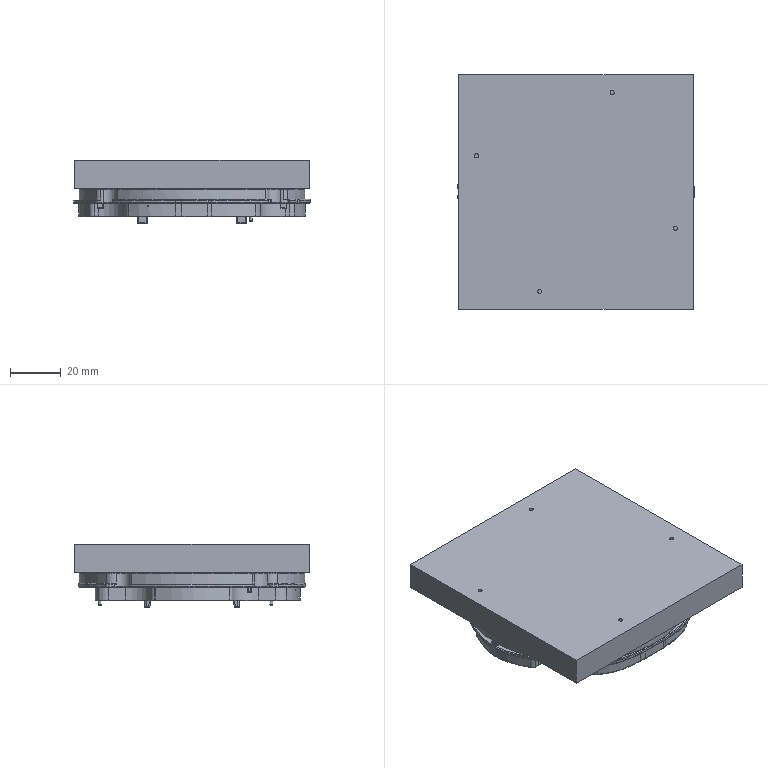NC program | NX | posted with a generic post | part box 92.935 x 92.1 x 24.829 mm
Lines 11819 to 12564 of 39008:
(ADAPTIVE_MILLING_COPY , TOOL : D3-9-D4-50-3T-ROUGH)
N23624 T15 M6
N23626 G54
N23628 G17 G0 G90 X32.559 Y-28.253 S5500 M3
N23630 G43 Z20. H15
N23632 Z-4.875
N23634 G94 G1 X32.611 Y-28.113 Z-5.812 F3000.
N23636 X32.662 Y-27.972 Z-6.183
N23638 X32.714 Y-27.831 Z-6.456
N23640 X32.765 Y-27.69 Z-6.675
N23642 X32.817 Y-27.549 Z-6.86
N23644 X32.868 Y-27.408 Z-7.018
N23646 X32.92 Y-27.267 Z-7.155
N23648 X32.971 Y-27.126 Z-7.275
N23650 X33.023 Y-26.986 Z-7.381
N23652 X33.074 Y-26.845 Z-7.474
N23654 X33.126 Y-26.704 Z-7.555
N23656 X33.177 Y-26.563 Z-7.625
N23658 X33.229 Y-26.422 Z-7.686
N23660 X33.28 Y-26.281 Z-7.737
N23662 X33.332 Y-26.14 Z-7.78
N23664 X33.383 Y-25.999 Z-7.815
N23666 X33.435 Y-25.858 Z-7.842
N23668 X33.486 Y-25.718 Z-7.86
N23670 X33.538 Y-25.577 Z-7.872
N23672 X33.589 Y-25.436 Z-7.875
N23674 X33.692 Y-25.162
N23676 X33.783 Y-24.884
N23678 G3 X33.696 Y-24.632 R0.309
N23680 X31.619 Y-23.863 R2.562
N23682 X28.424 Y-26.256 R3.555
N23684 G1 Y-26.893
N23686 G3 X28.606 Y-27.188 R0.332
N23688 X28.976 Y-27.152 Z-7.809 R0.385
N23690 G1 X29.156 Y-27.065 Z-7.775
N23692 X33.131 Y-25.119 F15000.
N23694 X33.313 Y-25.032 Z-7.81 F3000.
N23696 X33.488 Y-24.932 Z-7.844
N23698 X33.55 Y-24.863 Z-7.86
N23700 X33.591 Y-24.781 Z-7.875
N23702 G3 X33.511 Y-24.446 R0.332
N23704 X31.622 Y-23.664 R2.242
N23706 X28.444 Y-25.702 R3.596
N23708 G1 X28.424 Y-26.264
N23710 G3 X28.601 Y-26.556 R0.332
N23712 X28.967 Y-26.532 Z-7.811 R0.391
N23714 G1 X29.156 Y-26.449 Z-7.775
N23716 X32.857 Y-24.844 F15000.
N23718 X33.045 Y-24.764 Z-7.81 F3000.
N23720 X33.227 Y-24.672 Z-7.845
N23722 X33.29 Y-24.608 Z-7.86
N23724 X33.336 Y-24.531 Z-7.875
N23726 G3 X33.323 Y-24.259 R0.337
N23728 X32.298 Y-23.553 R1.442
N23730 X28.496 Y-25.188 R3.657
N23732 G1 X28.442 Y-25.733
N23734 G3 X28.594 Y-26.038 R0.332
N23736 X28.961 Y-26.042 Z-7.81 R0.39
N23738 G1 X29.156 Y-25.975 Z-7.775
N23740 X32.755 Y-24.735 F15000.
N23742 X32.955 Y-24.668 Z-7.811 F3000.
N23744 X33.15 Y-24.589 Z-7.847
N23746 X33.215 Y-24.536 Z-7.861
N23748 X33.266 Y-24.47 Z-7.875
N23750 G3 X33.272 Y-24.159 R0.334
N23752 X32.215 Y-23.363 R1.429
N23754 X28.532 Y-24.788 R3.673
N23756 G1 X28.478 Y-25.273
N23758 G3 X28.627 Y-25.575 R0.333
N23760 X28.979 Y-25.592 Z-7.813 R0.387
N23762 G1 X29.192 Y-25.53 Z-7.775
N23764 X32.625 Y-24.526 F15000.
N23766 X32.831 Y-24.467 Z-7.812 F3000.
N23768 X33.033 Y-24.398 Z-7.848
N23770 X33.097 Y-24.35 Z-7.862
N23772 X33.151 Y-24.29 Z-7.875
N23774 G3 X33.17 Y-23.959 R0.333
N23776 X32.084 Y-23.163 R1.454
N23778 X28.602 Y-24.38 R3.693
N23780 X28.51 Y-24.866 R2.637
N23782 X28.656 Y-25.166 R0.333
N23784 X29. Y-25.192 Z-7.815 R0.396
N23786 G1 X29.224 Y-25.138 Z-7.775
N23788 X32.533 Y-24.343 F15000.
N23790 X32.736 Y-24.296 Z-7.811 F3000.
N23792 X32.937 Y-24.236 Z-7.847
N23794 X33.007 Y-24.188 Z-7.861
N23796 X33.065 Y-24.126 Z-7.875
N23798 G3 X33.085 Y-23.791 R0.333
N23800 X32.027 Y-22.98 R1.401
N23802 X28.709 Y-23.971 R3.668
N23804 G1 X28.576 Y-24.446
N23806 G3 X28.686 Y-24.777 R0.332
N23808 X29.041 Y-24.831 Z-7.812 R0.382
N23810 G1 X29.252 Y-24.788 Z-7.775
N23812 X32.435 Y-24.153 F15000.
N23814 X32.643 Y-24.113 Z-7.811 F3000.
N23816 X32.849 Y-24.062 Z-7.848
N23818 X32.919 Y-24.019 Z-7.861
N23820 X32.978 Y-23.962 Z-7.875
N23822 G3 X33.043 Y-23.709 R0.339
N23824 X32.37 Y-22.942 R1.058
N23826 X29.652 Y-23.059 R3.291
N23828 X28.772 Y-23.665 R2.172
N23830 G1 X28.666 Y-24.071
N23832 G3 X28.766 Y-24.394 R0.333
N23834 X29.113 Y-24.464 Z-7.813 R0.386
N23836 G1 X29.332 Y-24.435 Z-7.775
N23838 X32.373 Y-24.026 F15000.
N23840 X32.598 Y-23.999 Z-7.814 F3000.
N23842 X32.821 Y-23.955 Z-7.853
N23844 X32.933 Y-23.882 Z-7.875
N23846 G3 X33.025 Y-23.598 R0.334
N23848 X32.262 Y-22.73 R1.156
N23850 X28.885 Y-23.292 R3.407
N23852 X28.746 Y-23.74 R1.548
N23854 X28.842 Y-24.059 R0.333
N23856 X29.178 Y-24.139 Z-7.815 R0.396
N23858 G1 X29.408 Y-24.121 Z-7.775
N23860 X32.327 Y-23.896 F15000.
N23862 X32.556 Y-23.882 Z-7.814 F3000.
N23864 X32.783 Y-23.851 Z-7.854
N23866 X32.896 Y-23.789 Z-7.875
N23868 G3 X33.008 Y-23.486 R0.333
N23870 X32.259 Y-22.565 R1.163
N23872 X29.043 Y-22.925 R3.351
N23874 X28.828 Y-23.4 R4.539
N23876 X28.918 Y-23.733 R0.319
N23878 X29.229 Y-23.811 Z-7.819 R0.389
N23880 G1 X29.486 Y-23.8 Z-7.775
N23882 X32.287 Y-23.684 F15000.
N23884 X32.52 Y-23.677 Z-7.815 F3000.
N23886 X32.751 Y-23.655 Z-7.855
N23888 X32.861 Y-23.6 Z-7.875
N23890 G3 X32.978 Y-23.301 R0.32
N23892 X32.217 Y-22.377 R1.206
N23894 X29.175 Y-22.613 R3.245
N23896 X28.99 Y-23.002 R3.691
N23898 X29.038 Y-23.336 R0.333
N23900 X29.37 Y-23.46 Z-7.813 R0.386
N23902 G1 X29.59 Y-23.465 Z-7.775
N23904 X32.262 Y-23.526 F15000.
N23906 X32.476 Y-23.533 Z-7.812 F3000.
N23908 X32.69 Y-23.528 Z-7.848
N23910 X32.766 Y-23.503 Z-7.862
N23912 X32.835 Y-23.463 Z-7.875
N23914 G3 X32.955 Y-23.153 R0.333
N23916 X32.258 Y-22.229 R1.165
N23918 X29.304 Y-22.319 R3.114
N23920 X29.106 Y-22.721 R1.623
N23922 X29.152 Y-23.052 R0.333
N23924 X29.474 Y-23.182 Z-7.814 R0.393
N23926 G1 X29.702 Y-23.197 Z-7.775
N23928 X32.237 Y-23.366 F15000.
N23930 X32.45 Y-23.382 Z-7.812 F3000.
N23932 X32.663 Y-23.387 Z-7.848
N23934 X32.741 Y-23.364 Z-7.862
N23936 X32.812 Y-23.327 Z-7.875
N23938 G3 X32.946 Y-23.061 R0.335
N23940 X32.403 Y-22.149 R1.061
N23942 X29.455 Y-22.026 R3.026
N23944 X29.233 Y-22.415 R0.964
N23946 X29.276 Y-22.743 R0.333
N23948 X29.58 Y-22.879 Z-7.817 R0.393
N23950 G1 X29.823 Y-22.908 Z-7.775
N23952 X32.212 Y-23.195 F15000.
N23954 X32.438 Y-23.225 Z-7.814 F3000.
N23956 X32.665 Y-23.237 Z-7.853
N23958 X32.789 Y-23.192 Z-7.875
N23960 G3 X32.946 Y-22.911 R0.333
N23962 X32.373 Y-21.954 R1.113
N23964 X29.613 Y-21.755 R2.886
N23966 G1 X29.378 Y-22.103
N23968 G3 X29.389 Y-22.465 R0.332
N23970 X29.687 Y-22.614 Z-7.817 R0.392
N23972 G1 X29.928 Y-22.654 Z-7.775
N23974 X32.203 Y-23.027 F15000.
N23976 X32.416 Y-23.064 Z-7.812 F3000.
N23978 X32.63 Y-23.09 Z-7.849
N23980 X32.707 Y-23.076 Z-7.862
N23982 X32.78 Y-23.047 Z-7.875
N23984 G3 X32.946 Y-22.761 R0.333
N23986 X32.363 Y-21.77 R1.152
N23988 X29.804 Y-21.477 R2.856
N23990 X29.551 Y-21.821 R1.132
N23992 X29.544 Y-22.154 R0.333
N23994 X29.844 Y-22.334 Z-7.814 R0.391
N23996 G1 X30.065 Y-22.383 Z-7.775
N23998 X32.204 Y-22.857 F15000.
N24000 X32.409 Y-22.905 Z-7.811 F3000.
N24002 X32.616 Y-22.94 Z-7.847
N24004 X32.699 Y-22.928 Z-7.861
N24006 X32.777 Y-22.899 Z-7.875
N24008 G3 X32.946 Y-22.611 R0.333
N24010 X32.355 Y-21.583 R1.175
N24012 X29.962 Y-21.237 R2.722
N24014 X29.692 Y-21.591 R0.912
N24016 X29.684 Y-21.923 R0.333
N24018 X29.978 Y-22.104 Z-7.815 R0.396
N24020 G1 X30.202 Y-22.16 Z-7.775
N24022 X32.204 Y-22.66 F15000.
N24024 X32.405 Y-22.713 Z-7.811 F3000.
N24026 X32.61 Y-22.752 Z-7.846
N24028 X32.695 Y-22.742 Z-7.861
N24030 X32.776 Y-22.712 Z-7.875
N24032 G3 X32.946 Y-22.423 R0.333
N24034 X32.367 Y-21.408 R1.195
N24036 X30.107 Y-21.014 R2.587
N24038 X29.845 Y-21.341 R0.773
N24040 X29.836 Y-21.67 R0.333
N24042 X30.109 Y-21.853 Z-7.818 R0.396
N24044 G1 X30.347 Y-21.926 Z-7.775
N24046 X32.205 Y-22.493 F15000.
N24048 X32.399 Y-22.554 Z-7.81 F3000.
N24050 X32.597 Y-22.602 Z-7.845
N24052 X32.687 Y-22.594 Z-7.86
N24054 X32.772 Y-22.564 Z-7.875
N24056 G3 X32.946 Y-22.273 R0.333
N24058 X32.375 Y-21.229 R1.214
N24060 X30.29 Y-20.79 R2.481
N24062 X29.976 Y-21.127 R1.274
N24064 X29.965 Y-21.452 R0.333
N24066 X30.237 Y-21.639 Z-7.818 R0.396
N24068 G1 X30.474 Y-21.713 Z-7.775
N24070 X32.201 Y-22.259 F15000.
N24072 X32.396 Y-22.323 Z-7.81 F3000.
N24074 X32.596 Y-22.374 Z-7.845
N24076 X32.684 Y-22.368 Z-7.86
N24078 X32.768 Y-22.341 Z-7.875
N24080 G3 X32.946 Y-22.097 R0.334
N24082 X32.493 Y-21.135 R1.104
N24084 X30.486 Y-20.578 R2.377
N24086 X30.171 Y-20.883 R1.01
N24088 X30.115 Y-21.217 R0.333
N24090 X30.381 Y-21.436 Z-7.815 R0.396
N24092 G1 X30.596 Y-21.521 Z-7.775
N24094 X32.204 Y-22.157 F15000.
N24096 X32.393 Y-22.234 Z-7.81 F3000.
N24098 X32.586 Y-22.297 Z-7.845
N24100 X32.676 Z-7.86
N24102 X32.764 Y-22.274 Z-7.875
N24104 G3 X32.958 Y-22.023 R0.334
N24106 X32.513 Y-20.958 R1.122
N24108 X30.655 Y-20.387 R2.237
N24110 X30.357 Y-20.665 R0.865
N24112 X30.297 Y-20.989 R0.333
N24114 X30.544 Y-21.213 Z-7.817 R0.391
N24116 G1 X30.765 Y-21.315 Z-7.775
N24118 X32.214 Y-21.983 F15000.
N24120 X32.399 Y-22.071 Z-7.81 F3000.
N24122 X32.59 Y-22.146 Z-7.845
N24124 X32.679 Y-22.151 Z-7.86
N24126 X32.766 Y-22.134 Z-7.875
N24128 G3 X32.982 Y-21.875 R0.333
N24130 X32.558 Y-20.801 R1.137
N24132 X30.797 Y-20.214 R2.071
N24134 X30.506 Y-20.491 R0.946
N24136 X30.444 Y-20.809 R0.333
N24138 X30.682 Y-21.037 Z-7.818 R0.395
N24140 G1 X30.903 Y-21.149 Z-7.775
N24142 X32.236 Y-21.821 F15000.
N24144 X32.416 Y-21.915 Z-7.81 F3000.
N24146 X32.604 Y-21.995 Z-7.845
N24148 X32.693 Y-22.003 Z-7.86
N24150 X32.782 Y-21.989 Z-7.875
N24152 G3 X33.005 Y-21.727 R0.332
N24154 X32.621 Y-20.661 R1.127
N24156 X30.974 Y-20.037 R1.999
N24158 X30.672 Y-20.297 R0.667
N24160 X30.609 Y-20.614 R0.333
N24162 X30.839 Y-20.842 Z-7.819 R0.403
N24164 G1 X31.063 Y-20.964 Z-7.775
N24166 X32.267 Y-21.625 F15000.
N24168 X32.442 Y-21.723 Z-7.81 F3000.
N24170 X32.624 Y-21.808 Z-7.844
N24172 X32.717 Y-21.818 Z-7.86
N24174 X32.809 Y-21.804 Z-7.875
N24176 G3 X33.034 Y-21.542 R0.332
N24178 X32.651 Y-20.486 R1.133
N24180 X31.124 Y-19.883 R1.838
N24182 X30.814 Y-20.13 R1.639
N24184 X30.751 Y-20.446 R0.333
N24186 X30.973 Y-20.673 Z-7.82 R0.41
N24188 G1 X31.199 Y-20.807 Z-7.775
N24190 X32.295 Y-21.454 F15000.
N24192 X32.47 Y-21.559 Z-7.81 F3000.
N24194 X32.652 Y-21.653 Z-7.845
N24196 X32.74 Y-21.666 Z-7.86
N24198 X32.829 Y-21.658 Z-7.875
N24200 G3 X33.043 Y-21.488 R0.337
N24202 X32.867 Y-20.531 R0.939
N24204 X31.333 Y-19.725 R1.838
N24206 X31.009 Y-19.951 R1.02
N24208 X30.902 Y-20.276 R0.332
N24210 X31.108 Y-20.522 Z-7.819 R0.406
N24212 G1 X31.321 Y-20.668 Z-7.775
N24214 X32.315 Y-21.351 F15000.
N24216 X32.485 Y-21.47 Z-7.811 F3000.
N24218 X32.662 Y-21.578 Z-7.846
N24220 X32.747 Y-21.598 Z-7.861
N24222 X32.833 Z-7.875
N24224 G3 X33.077 Y-21.421 R0.334
N24226 X32.957 Y-20.428 R0.95
N24228 X31.494 Y-19.588 R1.734
N24230 X31.198 Y-19.79 R0.966
N24232 X31.086 Y-20.09 R0.333
N24234 X31.274 Y-20.352 Z-7.819 R0.404
N24236 G1 X31.475 Y-20.512 Z-7.775
N24238 X32.354 Y-21.211 F15000.
N24240 X32.518 Y-21.344 Z-7.811 F3000.
N24242 X32.689 Y-21.467 Z-7.847
N24244 X32.768 Y-21.493 Z-7.861
N24246 X32.851 Y-21.501 Z-7.875
N24248 G3 X33.128 Y-21.321 R0.333
N24250 X32.991 Y-20.235 R1.01
N24252 X31.651 Y-19.459 R1.632
N24254 X31.345 Y-19.663 R0.885
N24256 X31.233 Y-19.962 R0.333
N24258 X31.425 Y-20.235 Z-7.817 R0.448
N24260 G1 X31.611 Y-20.397 Z-7.775
N24262 X32.409 Y-21.093 F15000.
N24264 X32.565 Y-21.232 Z-7.811 F3000.
N24266 X32.729 Y-21.361 Z-7.846
N24268 X32.809 Y-21.39 Z-7.861
N24270 X32.894 Y-21.401 Z-7.875
N24272 G3 X33.179 Y-21.221 R0.333
N24274 X33.086 Y-20.135 R1.021
N24276 X31.826 Y-19.334 R1.595
N24278 X31.515 Y-19.518 R0.627
N24280 X31.403 Y-19.816 R0.333
N24282 X31.584 Y-20.087 Z-7.819 R0.465
N24284 G1 X31.769 Y-20.263 Z-7.775
N24286 X32.484 Y-20.946 F15000.
N24288 X32.631 Y-21.089 Z-7.81 F3000.
N24290 X32.787 Y-21.221 Z-7.845
N24292 X32.87 Y-21.255 Z-7.86
N24294 X32.958 Y-21.267 Z-7.875
N24296 G3 X33.247 Y-21.087 R0.332
N24298 X33.157 Y-19.99 R1.03
N24300 X31.949 Y-19.219 R1.495
N24302 X31.653 Y-19.4 R0.683
N24304 X31.541 Y-19.7 R0.333
N24306 X31.73 Y-19.971 Z-7.818 R0.454
N24308 G1 X31.917 Y-20.138 Z-7.775
N24310 X32.589 Y-20.74 F15000.
N24312 X32.745 Y-20.881 Z-7.811 F3000.
N24314 X32.908 Y-21.014 Z-7.847
N24316 X32.986 Y-21.044 Z-7.861
N24318 X33.069 Y-21.057 Z-7.875
N24320 G3 X33.323 Y-20.937 R0.336
N24322 X33.31 Y-19.997 R0.927
N24324 X32.126 Y-19.107 R1.494
N24326 X31.769 Y-19.302 R0.833
N24328 X31.657 Y-19.6 R0.333
N24330 X31.821 Y-19.861 Z-7.822 R0.468
N24332 G1 X32.011 Y-20.058 Z-7.775
N24334 X32.617 Y-20.688 F15000.
N24336 X32.759 Y-20.839 Z-7.811 F3000.
N24338 X32.91 Y-20.98 Z-7.846
N24340 X32.989 Y-21.016 Z-7.861
N24342 X33.074 Y-21.034 Z-7.875
N24344 G3 X33.323 Y-20.937 R0.338
N24346 X33.455 Y-20.019 R0.834
N24348 X32.297 Y-19.007 R1.462
N24350 X31.97 Y-19.16 R0.936
N24352 X31.813 Y-19.469 R0.332
N24354 X31.97 Y-19.746 Z-7.82 R0.479
N24356 G1 X32.142 Y-19.945 Z-7.775
N24358 X32.681 Y-20.565 F15000.
N24360 X32.822 Y-20.729 Z-7.812 F3000.
N24362 X32.97 Y-20.886 Z-7.849
N24364 X33.038 Y-20.925 Z-7.862
N24366 X33.112 Y-20.95 Z-7.875
N24368 G3 X33.403 Y-20.858 R0.334
N24370 X33.532 Y-19.867 R0.897
N24372 X32.455 Y-18.914 R1.397
N24374 X32.151 Y-19.049 R0.837
N24376 X31.993 Y-19.327 R0.333
N24378 X32.125 Y-19.619 Z-7.82 R0.477
N24380 G1 X32.279 Y-19.831 Z-7.775
N24382 X32.745 Y-20.474 F15000.
N24384 X32.869 Y-20.648 Z-7.812 F3000.
N24386 X33.002 Y-20.816 Z-7.848
N24388 X33.068 Y-20.861 Z-7.862
N24390 X33.142 Y-20.892 Z-7.875
N24392 G3 X33.456 Y-20.805 R0.333
N24394 X33.646 Y-19.81 R0.901
N24396 X32.592 Y-18.824 R1.348
N24398 X32.301 Y-18.957 R0.968
N24400 X32.144 Y-19.232 R0.334
N24402 X32.27 Y-19.523 Z-7.82 R0.482
N24404 G1 X32.422 Y-19.74 Z-7.775
N24406 X32.852 Y-20.358 F15000.
N24408 X32.973 Y-20.535 Z-7.812 F3000.
N24410 X33.103 Y-20.705 Z-7.848
N24412 X33.168 Y-20.751 Z-7.862
N24414 X33.241 Y-20.784 Z-7.875
N24416 G3 X33.562 Y-20.699 R0.333
N24418 X33.728 Y-19.651 R0.949
N24420 X32.762 Y-18.739 R1.326
N24422 X32.44 Y-18.872 R0.675
N24424 X32.283 Y-19.147 R0.334
N24426 X32.397 Y-19.427 Z-7.823 R0.484
N24428 G1 X32.549 Y-19.663 Z-7.775
N24430 X32.941 Y-20.27 F15000.
N24432 X33.054 Y-20.448 Z-7.811 F3000.
N24434 X33.177 Y-20.62 Z-7.847
N24436 X33.243 Y-20.669 Z-7.861
N24438 X33.318 Y-20.703 Z-7.875
N24440 G3 X33.642 Y-20.619 R0.333
N24442 X33.84 Y-19.584 R0.946
N24444 X32.887 Y-18.656 R1.268
N24446 X32.575 Y-18.789 R0.733
N24448 X32.417 Y-19.065 R0.334
N24450 X32.53 Y-19.343 Z-7.824 R0.489
N24452 G1 X32.681 Y-19.583 Z-7.775
N24454 X33.049 Y-20.162 F15000.
N24456 X33.16 Y-20.34 Z-7.811 F3000.
N24458 X33.281 Y-20.512 Z-7.847
N24460 X33.348 Y-20.563 Z-7.861
N24462 X33.424 Y-20.597 Z-7.875
N24464 G3 X33.748 Y-20.513 R0.333
N24466 X33.933 Y-19.452 R0.96
N24468 X33.024 Y-18.575 R1.236
N24470 X32.708 Y-18.708 R0.701
N24472 X32.55 Y-18.984 R0.333
N24474 X32.657 Y-19.259 Z-7.825 R0.505
N24476 G1 X32.806 Y-19.507 Z-7.775
N24478 X33.143 Y-20.068 F15000.
N24480 X33.252 Y-20.252 Z-7.812 F3000.
N24482 X33.37 Y-20.431 Z-7.848
N24484 X33.432 Y-20.481 Z-7.862
N24486 X33.503 Y-20.518 Z-7.875
N24488 G3 X33.76 Y-20.501 R0.34
N24490 X34.107 Y-19.671 R0.799
N24492 X33.182 Y-18.5 R1.285
N24494 X32.838 Y-18.628 R0.69
N24496 X32.68 Y-18.906 R0.333
N24498 X32.785 Y-19.189 Z-7.824 R0.61
N24500 G1 X32.917 Y-19.44 Z-7.775
N24502 X33.213 Y-19.999 F15000.
N24504 X33.316 Y-20.2 Z-7.814 F3000.
N24506 X33.433 Y-20.393 Z-7.852
N24508 X33.485 Y-20.437 Z-7.864
N24510 X33.543 Y-20.474 Z-7.875
N24512 G3 X33.827 Y-20.467 R0.336
N24514 X34.22 Y-19.609 R0.832
N24516 X33.363 Y-18.435 R1.299
N24518 X33.041 Y-18.521 R0.831
N24520 X32.838 Y-18.814 R0.332
N24522 G1 X32.866 Y-18.958 Z-7.851
N24524 X32.925 Y-19.093 Z-7.826
N24526 X33.043 Y-19.363 Z-7.775
N24528 X33.291 Y-19.928 F15000.
N24530 X33.38 Y-20.137 Z-7.814 F3000.
N24532 X33.484 Y-20.339 Z-7.853
N24534 X33.584 Y-20.427 Z-7.875
N24536 G3 X33.894 Y-20.432 R0.334
N24538 X34.335 Y-19.551 R0.853
N24540 X33.515 Y-18.374 R1.268
N24542 X33.192 Y-18.458 R0.789
N24544 X32.99 Y-18.729 R0.333
N24546 X33.065 Y-19.018 Z-7.824 R0.626
N24548 G1 X33.171 Y-19.285 Z-7.775
N24550 X33.397 Y-19.855 F15000.
N24552 X33.479 Y-20.069 Z-7.814 F3000.
N24554 X33.576 Y-20.277 Z-7.853
N24556 X33.669 Y-20.367 Z-7.875
N24558 G3 X33.994 Y-20.381 R0.333
N24560 X34.449 Y-19.434 R0.893
N24562 X33.67 Y-18.316 R1.247
N24564 X33.337 Y-18.398 R0.703
N24566 X33.138 Y-18.648 R0.333
N24568 X33.2 Y-18.947 Z-7.823 R0.584
N24570 G1 X33.295 Y-19.21 Z-7.775
N24572 X33.507 Y-19.797 F15000.
N24574 X33.582 Y-20.011 Z-7.814 F3000.
N24576 X33.672 Y-20.22 Z-7.853
N24578 X33.766 Y-20.314 Z-7.875
N24580 G3 X34.094 Y-20.33 R0.333
N24582 X34.568 Y-19.359 R0.908
N24584 X33.823 Y-18.26 R1.24
N24586 X33.51 Y-18.326 R0.612
N24588 X33.311 Y-18.575 R0.333
N24590 X33.368 Y-18.87 Z-7.824 R0.615
N24592 G1 X33.457 Y-19.141 Z-7.775
N24594 X33.65 Y-19.724 F15000.
N24596 X33.718 Y-19.941 Z-7.814 F3000.
N24598 X33.804 Y-20.152 Z-7.853
N24600 X33.899 Y-20.245 Z-7.875
N24602 G3 X34.228 Y-20.262 R0.333
N24604 X34.69 Y-19.305 R0.92
N24606 X33.951 Y-18.201 R1.205
N24608 X33.615 Y-18.283 R0.69
N24610 X33.416 Y-18.53 R0.334
N24612 X33.478 Y-18.818 Z-7.825 R0.506
N24614 G1 X33.586 Y-19.087 Z-7.775
N24616 X33.808 Y-19.643 F15000.
N24618 X33.893 Y-19.863 Z-7.816 F3000.
N24620 X33.991 Y-20.078 Z-7.856
N24622 X34.071 Y-20.162 Z-7.875
N24624 G3 X34.311 Y-20.22 R0.342
N24626 X34.808 Y-19.489 R0.801
N24628 X34.103 Y-18.147 R1.257
N24630 X33.784 Y-18.213 R0.592
N24632 X33.584 Y-18.466 R0.333
N24634 G1 X33.594 Y-18.618 Z-7.85
N24636 X33.632 Y-18.765 Z-7.824
N24638 X33.702 Y-19.041 Z-7.775
N24640 X33.85 Y-19.623 F15000.
N24642 X33.902 Y-19.832 Z-7.812 F3000.
N24644 X33.963 Y-20.038 Z-7.849
N24646 X34.007 Y-20.104 Z-7.862
N24648 X34.063 Y-20.159 Z-7.875
N24650 G3 X34.311 Y-20.22 R0.34
N24652 X34.913 Y-19.55 R0.757
N24654 X34.277 Y-18.103 R1.301
N24656 X33.918 Y-18.157 R0.489
N24658 X33.718 Y-18.413 R0.333
N24660 G1 X33.727 Y-18.562 Z-7.85
N24662 X33.762 Y-18.706 Z-7.825
N24664 X33.827 Y-18.99 Z-7.775
N24666 X33.96 Y-19.567 F15000.
N24668 X34.011 Y-19.795 Z-7.815 F3000.
N24670 X34.074 Y-20.019 Z-7.855
N24672 X34.145 Y-20.118 Z-7.875
N24674 G3 X34.422 Y-20.202 R0.335
N24676 X35.054 Y-19.435 R0.836
N24678 X34.402 Y-18.047 R1.283
N24680 X34.031 Y-18.11 R0.584
N24682 X33.831 Y-18.369 R0.333
N24684 G1 X33.843 Y-18.537 Z-7.847
N24686 X33.878 Y-18.7 Z-7.819
N24688 X33.927 Y-18.949 Z-7.775
N24690 X34.042 Y-19.532 F15000.
N24692 X34.086 Y-19.765 Z-7.816 F3000.
N24694 X34.142 Y-19.995 Z-7.856
N24696 X34.204 Y-20.091 Z-7.875
N24698 G3 X34.496 Y-20.191 R0.334
N24700 X35.166 Y-19.484 R0.827
N24702 X34.569 Y-18.009 R1.31
N24704 X34.234 Y-18.04 R0.746
N24706 X33.985 Y-18.309 R0.332
N24708 G1 X33.993 Y-18.475 Z-7.847
N24710 X34.022 Y-18.639 Z-7.819
N24712 X34.064 Y-18.892 Z-7.775
N24714 X34.163 Y-19.495 F15000.
N24716 X34.2 Y-19.731 Z-7.816 F3000.
N24718 X34.248 Y-19.965 Z-7.857
N24720 X34.304 Y-20.06 Z-7.875
N24722 G3 X34.607 Y-20.173 R0.333
N24724 X35.306 Y-19.409 R0.87
N24726 X34.76 Y-17.987 R1.336
N24728 X34.385 Y-18.003 R0.564
N24730 X34.14 Y-18.252 R0.332
N24732 G1 X34.139 Y-18.407 Z-7.849
N24734 X34.161 Y-18.561 Z-7.823
N24736 X34.199 Y-18.837 Z-7.775
N24738 X34.285 Y-19.473 F15000.
N24740 X34.315 Y-19.708 Z-7.816 F3000.
N24742 X34.357 Y-19.941 Z-7.856
N24744 X34.413 Y-20.041 Z-7.875
N24746 G3 X34.718 Y-20.156 R0.333
N24748 X35.441 Y-19.37 R0.898
N24750 X34.898 Y-17.946 R1.318
N24752 X34.531 Y-17.968 R0.613
N24754 X34.291 Y-18.197 R0.333
N24756 G1 X34.282 Y-18.347 Z-7.85
N24758 X34.3 Y-18.497 Z-7.824
N24760 X34.331 Y-18.782 Z-7.775
N24762 X34.406 Y-19.454 F15000.
N24764 X34.43 Y-19.687 Z-7.815 F3000.
N24766 X34.467 Y-19.919 Z-7.855
N24768 X34.524 Y-20.023 Z-7.875
N24770 G3 X34.829 Y-20.138 R0.333
N24772 X35.559 Y-19.409 R0.89
N24774 X35.043 Y-17.908 R1.324
N24776 X34.682 Y-17.932 R0.625
N24778 X34.445 Y-18.149 R0.333
N24780 G1 X34.431 Y-18.302 Z-7.849
N24782 X34.448 Y-18.455 Z-7.823
N24784 X34.478 Y-18.734 Z-7.775
N24786 X34.552 Y-19.431 F15000.
N24788 X34.575 Y-19.665 Z-7.815 F3000.
N24790 X34.61 Y-19.898 Z-7.855
N24792 X34.666 Y-20.002 Z-7.875
N24794 G3 X34.922 Y-20.123 R0.336
N24796 X35.651 Y-19.516 R0.834
N24798 X35.236 Y-17.897 R1.382
N24800 X34.831 Y-17.896 R0.499
N24802 X34.593 Y-18.118 R0.333
N24804 G1 X34.579 Y-18.279 Z-7.848
N24806 X34.59 Y-18.441 Z-7.82
N24808 X34.605 Y-18.705 Z-7.775
N24810 X34.646 Y-19.417 F15000.
N24812 X34.656 Y-19.651 Z-7.815 F3000.
N24814 X34.681 Y-19.883 Z-7.855
N24816 X34.734 Y-19.991 Z-7.875
N24818 G3 X34.997 Y-20.123 R0.335
N24820 X35.79 Y-19.507 R0.863
N24822 X35.371 Y-17.856 R1.386
N24824 X35.008 Y-17.853 R0.489
N24826 X34.769 Y-18.08 R0.333
N24828 G1 X34.754 Y-18.258 Z-7.845
N24830 X34.759 Y-18.438 Z-7.814
N24832 X34.763 Y-18.668 Z-7.775
N24834 X34.774 Y-19.397 F15000.
N24836 X34.775 Y-19.633 Z-7.816 F3000.
N24838 X34.789 Y-19.868 Z-7.856
N24840 X34.835 Y-19.976 Z-7.875
N24842 G3 X35.11 Y-20.123 R0.334
N24844 X35.962 Y-19.423 R0.919
N24846 X35.529 Y-17.828 R1.404
N24848 X35.121 Y-17.826 R0.496
N24850 X34.882 Y-18.053 R0.333
N24852 G1 X34.867 Y-18.232 Z-7.845
N24854 X34.872 Y-18.411 Z-7.815
N24856 X34.876 Y-18.641 Z-7.775
N24858 X34.886 Y-19.386 F15000.
N24860 X34.888 Y-19.625 Z-7.816 F3000.
N24862 X34.901 Y-19.864 Z-7.857
N24864 X34.941 Y-19.966 Z-7.875
N24866 G3 X35.222 Y-20.123 R0.333
N24868 X36.114 Y-19.397 R0.948
N24870 X35.687 Y-17.801 R1.422
N24872 X35.291 Y-17.785 R0.491
N24874 X35.05 Y-18.017 R0.333
N24876 G1 X35.031 Y-18.268 Z-7.833
N24878 X35.03 Y-18.521 Z-7.79
N24880 X35.028 Y-18.605 Z-7.775
N24882 X35.013 Y-19.383 F15000.
N24884 X35.006 Y-19.62 Z-7.816 F3000.
N24886 X35.012 Y-19.856 Z-7.856
N24888 X35.052 Y-19.964 Z-7.875
N24890 G3 X35.335 Y-20.123 R0.333
N24892 X36.256 Y-19.41 R0.955
N24894 X35.835 Y-17.77 R1.428
N24896 X35.498 Y-17.748 R0.746
N24898 X35.209 Y-17.979 R0.332
N24900 G1 X35.189 Y-18.185 Z-7.84
N24902 X35.187 Y-18.391 Z-7.805
N24904 X35.183 Y-18.567 Z-7.775
N24906 X35.164 Y-19.382 F15000.
N24908 X35.157 Y-19.618 Z-7.816 F3000.
N24910 X35.162 Y-19.855 Z-7.856
N24912 X35.202 Y-19.963 Z-7.875
N24914 G3 X35.485 Y-20.123 R0.333
N24916 X36.407 Y-19.404 R0.964
N24918 X36.013 Y-17.761 R1.438
N24920 X35.667 Y-17.734 R0.684
N24922 X35.387 Y-17.942 R0.332
N24924 G1 X35.359 Y-18.108 Z-7.847
N24926 X35.356 Y-18.276 Z-7.818
N24928 X35.348 Y-18.528 Z-7.775
N24930 X35.319 Y-19.382 F15000.
N24932 X35.309 Y-19.617 Z-7.815 F3000.
N24934 X35.311 Y-19.853 Z-7.856
N24936 X35.352 Y-19.963 Z-7.875
N24938 G3 X35.635 Y-20.123 R0.333
N24940 X36.269 Y-20.032 R11.662
N24942 G2 X37.532 Y-20.22 R36.897
N24944 X38.519 Y-20.937 R2.29
N24946 G3 X39.067 Y-21.819 R3.155
N24948 X39.553 Y-21.533 R0.303
N24950 G1 X39.529 Y-21.385 Z-7.872
N24952 X39.506 Y-21.237 Z-7.86
N24954 X39.482 Y-21.089 Z-7.842
N24956 X39.459 Y-20.941 Z-7.815
N24958 X39.435 Y-20.793 Z-7.78
N24960 X39.412 Y-20.644 Z-7.737
N24962 X39.389 Y-20.496 Z-7.686
N24964 X39.365 Y-20.348 Z-7.625
N24966 X39.342 Y-20.2 Z-7.555
N24968 X39.318 Y-20.052 Z-7.474
N24970 X39.295 Y-19.904 Z-7.381
N24972 X39.271 Y-19.756 Z-7.275
N24974 X39.248 Y-19.607 Z-7.155
N24976 X39.225 Y-19.459 Z-7.018
N24978 X39.201 Y-19.311 Z-6.86
N24980 X39.178 Y-19.163 Z-6.675
N24982 X39.154 Y-19.015 Z-6.456
N24984 X39.131 Y-18.867 Z-6.183
N24986 X39.108 Y-18.718 Z-5.812
N24988 X39.084 Y-18.57 Z-4.875
N24990 G0 Z20.
N24992 X38.474 Y-19.387
N24994 Z-4.875
N24996 G1 X38.324 Z-5.812
N24998 X38.174 Z-6.183
N25000 X38.024 Z-6.456
N25002 X37.874 Z-6.675
N25004 X37.724 Z-6.86
N25006 X37.574 Z-7.018
N25008 X37.424 Z-7.155
N25010 X37.274 Z-7.275
N25012 X37.124 Z-7.381
N25014 X36.974 Z-7.474
N25016 X36.824 Z-7.555
N25018 X36.674 Z-7.625
N25020 X36.524 Z-7.686
N25022 X36.374 Z-7.737
N25024 X36.224 Z-7.78
N25026 X36.074 Z-7.815
N25028 X35.924 Z-7.842
N25030 X35.774 Z-7.86
N25032 X35.624 Z-7.872
N25034 X35.474 Z-7.875
N25036 G3 X35.343 Y-19.963 R0.303
N25038 X35.747 Y-20.123 R2.631
N25040 G1 X36.932 Y-20.108
N25042 X37.31 Y-19.869
N25044 X37.797 Y-19.538 Z-7.775
N25046 X39.984 Y-18.047 F15000.
N25048 X40.196 Y-17.907 Z-7.819 F3000.
N25050 X40.397 Y-17.752 Z-7.862
N25052 X40.444 Y-17.686 Z-7.875
N25054 G3 X39.977 Y-17.254 R0.33
N25056 X39.066 Y-17.91 R2.797
N25058 G2 X37.445 Y-18.023 R1.802
N25060 G3 X36.492 Y-17.669 R9.928
N25062 G1 X35.819 Y-17.722
N25064 G3 X35.634 Y-18.237 R0.3
N25066 X35.903 Y-18.35 Z-7.825 R0.6
N25068 G1 X36.186 Y-18.429 Z-7.775
N25070 X36.595 Y-18.54 F15000.
N25072 X39.904 Y-18.467
N25074 G3 X40.141 Y-18.226 R0.302
N25076 G1 X40.185 Y-17.987
N25078 X40.225 Y-17.782 Z-7.811 F3000.
N25080 X40.25 Y-17.576 Z-7.846
N25082 X40.231 Y-17.492 Z-7.861
N25084 X40.192 Y-17.416 Z-7.875
N25086 G3 X39.853 Y-17.312 R0.301
N25088 G2 X38.323 Y-17.651 R3.946
N25090 G3 X36.487 Y-17.67 R90.892
N25092 X36.252 Y-18.121 R0.3
N25094 X36.509 Y-18.288 Z-7.822 R0.429
N25096 G1 X36.767 Y-18.384 Z-7.775
N25098 X37.351 Y-18.599 F15000.
N25100 X37.425 Y-18.607
N25102 X38.882 Y-18.579
N25104 X38.947 Y-18.557
N25106 X39.008 Y-18.525
N25108 X39.36 Y-18.266